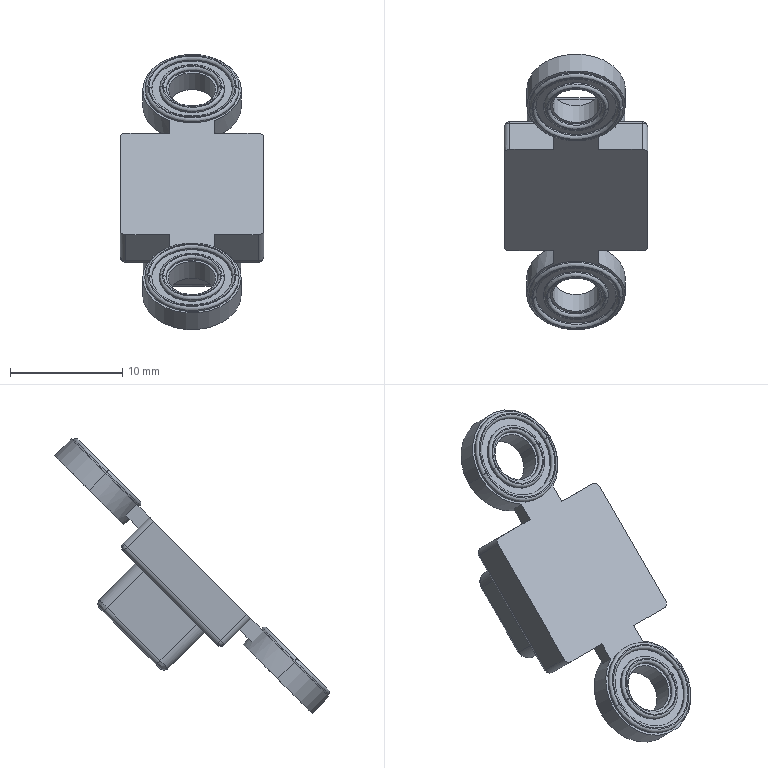Part | SolidWorks | features BaseBody 1 | 1 solid | 97 faces | box 12.809 x 24.563 x 24.582 mm | volume 1226 mm3 | cylinder 40 | plane 27 | torus 18 | sphere 8 | spline 4 | commonest cylinder face diameters 1 x12 2 x4 4.2 x4 4.62 x4 5.8 x4 7.2 x4